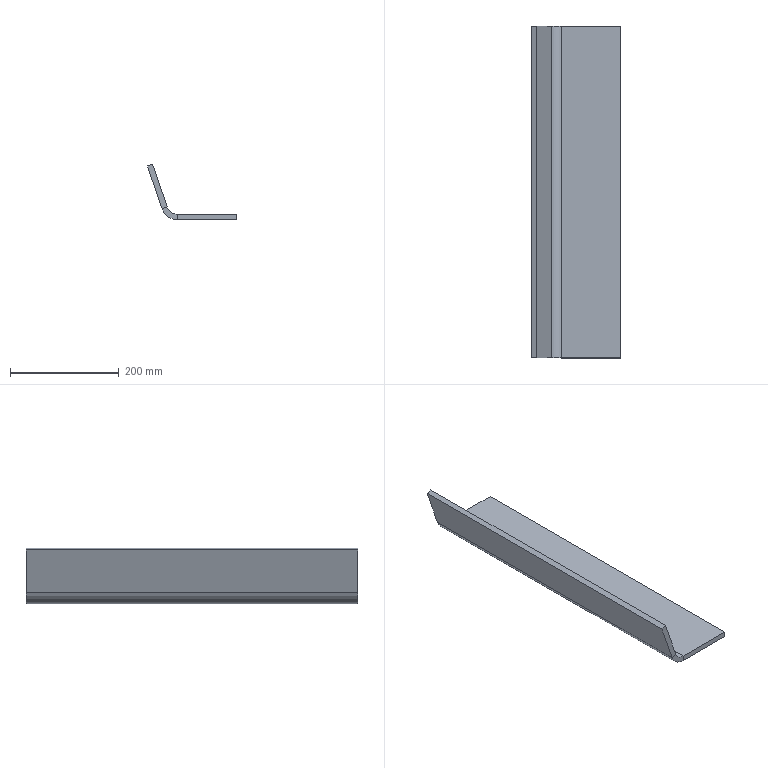Part | SolidWorks | features FlatPattern 1, SM3dBend 1, SMBaseFlange 1, SheetMetal 1 | 1 solid | 14 faces | box 163.637 x 610 x 102.048 mm | volume 1357250 mm3 | plane 12 | cylinder 2 | commonest cylinder face diameters 40 x1 60 x1
STEP:
#1=CARTESIAN_POINT('',(95.05,610.,13.555));
#2=VERTEX_POINT('',#1);
#3=CARTESIAN_POINT('',(68.329,610.,92.048));
#4=VERTEX_POINT('',#3);
#5=CARTESIAN_POINT('',(68.329,610.,92.048));
#6=DIRECTION('',(-0.3223,0.,0.9466));
#7=VECTOR('',#6,1000.);
#8=LINE('',#5,#7);
#9=EDGE_CURVE('',#2,#4,#8,.T.);
#10=ORIENTED_EDGE('',*,*,#9,.F.);
#11=CARTESIAN_POINT('',(85.584,610.,10.332));
#12=VERTEX_POINT('',#11);
#13=CARTESIAN_POINT('',(85.584,610.,10.332));
#14=DIRECTION('',(-0.9466,0.,-0.3223));
#15=VECTOR('',#14,1000.);
#16=LINE('',#13,#15);
#17=EDGE_CURVE('',#2,#12,#16,.T.);
#18=ORIENTED_EDGE('',*,*,#17,.T.);
#19=CARTESIAN_POINT('',(58.863,610.,88.825));
#20=VERTEX_POINT('',#19);
#21=CARTESIAN_POINT('',(58.863,610.,88.825));
#22=DIRECTION('',(-0.3223,0.,0.9466));
#23=VECTOR('',#22,1000.);
#24=LINE('',#21,#23);
#25=EDGE_CURVE('',#12,#20,#24,.T.);
#26=ORIENTED_EDGE('',*,*,#25,.T.);
#27=CARTESIAN_POINT('',(58.863,610.,88.825));
#28=DIRECTION('',(0.9466,0.,0.3223));
#29=VECTOR('',#28,1000.);
#30=LINE('',#27,#29);
#31=EDGE_CURVE('',#20,#4,#30,.T.);
#32=ORIENTED_EDGE('',*,*,#31,.T.);
#33=EDGE_LOOP('',(#10,#18,#26,#32));
#34=FACE_OUTER_BOUND('',#33,.T.);
#35=CARTESIAN_POINT('',(58.863,610.,88.825));
#36=DIRECTION('',(0.,1.,0.));
#37=DIRECTION('',(0.9466,0.,0.3223));
#38=AXIS2_PLACEMENT_3D('',#35,#36,#37);
#39=PLANE('',#38);
#40=ADVANCED_FACE('',(#34),#39,.T.);
#41=CARTESIAN_POINT('',(58.863,0.,88.825));
#42=VERTEX_POINT('',#41);
#43=CARTESIAN_POINT('',(85.584,0.,10.332));
#44=VERTEX_POINT('',#43);
#45=CARTESIAN_POINT('',(58.863,0.,88.825));
#46=DIRECTION('',(0.3223,0.,-0.9466));
#47=VECTOR('',#46,1000.);
#48=LINE('',#45,#47);
#49=EDGE_CURVE('',#42,#44,#48,.T.);
#50=ORIENTED_EDGE('',*,*,#49,.T.);
#51=CARTESIAN_POINT('',(95.05,0.,13.555));
#52=VERTEX_POINT('',#51);
#53=CARTESIAN_POINT('',(85.584,0.,10.332));
#54=DIRECTION('',(0.9466,0.,0.3223));
#55=VECTOR('',#54,1000.);
#56=LINE('',#53,#55);
#57=EDGE_CURVE('',#44,#52,#56,.T.);
#58=ORIENTED_EDGE('',*,*,#57,.T.);
#59=CARTESIAN_POINT('',(68.329,0.,92.048));
#60=VERTEX_POINT('',#59);
#61=CARTESIAN_POINT('',(68.329,0.,92.048));
#62=DIRECTION('',(0.3223,0.,-0.9466));
#63=VECTOR('',#62,1000.);
#64=LINE('',#61,#63);
#65=EDGE_CURVE('',#60,#52,#64,.T.);
#66=ORIENTED_EDGE('',*,*,#65,.F.);
#67=CARTESIAN_POINT('',(58.863,0.,88.825));
#68=DIRECTION('',(0.9466,0.,0.3223));
#69=VECTOR('',#68,1000.);
#70=LINE('',#67,#69);
#71=EDGE_CURVE('',#42,#60,#70,.T.);
#72=ORIENTED_EDGE('',*,*,#71,.F.);
#73=EDGE_LOOP('',(#50,#58,#66,#72));
#74=FACE_OUTER_BOUND('',#73,.T.);
#75=CARTESIAN_POINT('',(58.863,0.,88.825));
#76=DIRECTION('',(0.,-1.,0.));
#77=DIRECTION('',(-0.9466,0.,-0.3223));
#78=AXIS2_PLACEMENT_3D('',#75,#76,#77);
#79=PLANE('',#78);
#80=ADVANCED_FACE('',(#74),#79,.T.);
#81=ORIENTED_EDGE('',*,*,#25,.F.);
#82=CARTESIAN_POINT('',(85.584,610.,10.332));
#83=DIRECTION('',(0.,-1.,0.));
#84=VECTOR('',#83,1000.);
#85=LINE('',#82,#84);
#86=EDGE_CURVE('',#12,#44,#85,.T.);
#87=ORIENTED_EDGE('',*,*,#86,.T.);
#88=ORIENTED_EDGE('',*,*,#49,.F.);
#89=CARTESIAN_POINT('',(58.863,0.,88.825));
#90=DIRECTION('',(0.,-1.,0.));
#91=VECTOR('',#90,1000.);
#92=LINE('',#89,#91);
#93=EDGE_CURVE('',#20,#42,#92,.T.);
#94=ORIENTED_EDGE('',*,*,#93,.F.);
#95=EDGE_LOOP('',(#81,#87,#88,#94));
#96=FACE_OUTER_BOUND('',#95,.T.);
#97=CARTESIAN_POINT('',(58.863,610.,88.825));
#98=DIRECTION('',(-0.9466,0.,-0.3223));
#99=DIRECTION('',(-0.3223,0.,0.9466));
#100=AXIS2_PLACEMENT_3D('',#97,#98,#99);
#101=PLANE('',#100);
#102=ADVANCED_FACE('',(#96),#101,.T.);
#103=CARTESIAN_POINT('',(68.329,0.,92.048));
#104=DIRECTION('',(0.,-1.,0.));
#105=VECTOR('',#104,1000.);
#106=LINE('',#103,#105);
#107=EDGE_CURVE('',#4,#60,#106,.T.);
#108=ORIENTED_EDGE('',*,*,#107,.F.);
#109=ORIENTED_EDGE('',*,*,#31,.F.);
#110=ORIENTED_EDGE('',*,*,#93,.T.);
#111=ORIENTED_EDGE('',*,*,#71,.T.);
#112=EDGE_LOOP('',(#108,#109,#110,#111));
#113=FACE_OUTER_BOUND('',#112,.T.);
#114=CARTESIAN_POINT('',(58.863,0.,88.825));
#115=DIRECTION('',(-0.3223,0.,0.9466));
#116=DIRECTION('',(0.9466,0.,0.3223));
#117=AXIS2_PLACEMENT_3D('',#114,#115,#116);
#118=PLANE('',#117);
#119=ADVANCED_FACE('',(#113),#118,.T.);
#120=CARTESIAN_POINT('',(95.05,610.,13.555));
#121=DIRECTION('',(0.,-1.,0.));
#122=VECTOR('',#121,1000.);
#123=LINE('',#120,#122);
#124=EDGE_CURVE('',#2,#52,#123,.T.);
#125=ORIENTED_EDGE('',*,*,#124,.F.);
#126=ORIENTED_EDGE('',*,*,#9,.T.);
#127=ORIENTED_EDGE('',*,*,#107,.T.);
#128=ORIENTED_EDGE('',*,*,#65,.T.);
#129=EDGE_LOOP('',(#125,#126,#127,#128));
#130=FACE_OUTER_BOUND('',#129,.T.);
#131=CARTESIAN_POINT('',(68.329,610.,92.048));
#132=DIRECTION('',(-0.9466,0.,-0.3223));
#133=DIRECTION('',(-0.3223,0.,0.9466));
#134=AXIS2_PLACEMENT_3D('',#131,#132,#133);
#135=PLANE('',#134);
#136=ADVANCED_FACE('',(#130),#135,.F.);
#137=CARTESIAN_POINT('',(222.5,0.,0.));
#138=VERTEX_POINT('',#137);
#139=CARTESIAN_POINT('',(222.5,610.,0.));
#140=VERTEX_POINT('',#139);
#141=CARTESIAN_POINT('',(222.5,0.,0.));
#142=DIRECTION('',(0.,1.,0.));
#143=VECTOR('',#142,1000.);
#144=LINE('',#141,#143);
#145=EDGE_CURVE('',#138,#140,#144,.T.);
#146=ORIENTED_EDGE('',*,*,#145,.F.);
#147=CARTESIAN_POINT('',(222.5,0.,-10.));
#148=VERTEX_POINT('',#147);
#149=CARTESIAN_POINT('',(222.5,0.,-10.));
#150=DIRECTION('',(0.,0.,1.));
#151=VECTOR('',#150,1000.);
#152=LINE('',#149,#151);
#153=EDGE_CURVE('',#148,#138,#152,.T.);
#154=ORIENTED_EDGE('',*,*,#153,.F.);
#155=CARTESIAN_POINT('',(222.5,610.,-10.));
#156=VERTEX_POINT('',#155);
#157=CARTESIAN_POINT('',(222.5,0.,-10.));
#158=DIRECTION('',(0.,1.,0.));
#159=VECTOR('',#158,1000.);
#160=LINE('',#157,#159);
#161=EDGE_CURVE('',#148,#156,#160,.T.);
#162=ORIENTED_EDGE('',*,*,#161,.T.);
#163=CARTESIAN_POINT('',(222.5,610.,-10.));
#164=DIRECTION('',(0.,0.,1.));
#165=VECTOR('',#164,1000.);
#166=LINE('',#163,#165);
#167=EDGE_CURVE('',#156,#140,#166,.T.);
#168=ORIENTED_EDGE('',*,*,#167,.T.);
#169=EDGE_LOOP('',(#146,#154,#162,#168));
#170=FACE_OUTER_BOUND('',#169,.T.);
#171=CARTESIAN_POINT('',(222.5,0.,-10.));
#172=DIRECTION('',(1.,0.,0.));
#173=DIRECTION('',(0.,0.,-1.));
#174=AXIS2_PLACEMENT_3D('',#171,#172,#173);
#175=PLANE('',#174);
#176=ADVANCED_FACE('',(#170),#175,.T.);
#177=CARTESIAN_POINT('',(113.983,610.,-10.));
#178=VERTEX_POINT('',#177);
#179=CARTESIAN_POINT('',(113.983,0.,-10.));
#180=VERTEX_POINT('',#179);
#181=CARTESIAN_POINT('',(113.983,610.,-10.));
#182=DIRECTION('',(0.,-1.,0.));
#183=VECTOR('',#182,1000.);
#184=LINE('',#181,#183);
#185=EDGE_CURVE('',#178,#180,#184,.T.);
#186=ORIENTED_EDGE('',*,*,#185,.F.);
#187=CARTESIAN_POINT('',(0.,610.,-10.));
#188=DIRECTION('',(-1.,0.,0.));
#189=VECTOR('',#188,1000.);
#190=LINE('',#187,#189);
#191=EDGE_CURVE('',#156,#178,#190,.T.);
#192=ORIENTED_EDGE('',*,*,#191,.F.);
#193=ORIENTED_EDGE('',*,*,#161,.F.);
#194=CARTESIAN_POINT('',(0.,0.,-10.));
#195=DIRECTION('',(1.,0.,0.));
#196=VECTOR('',#195,1000.);
#197=LINE('',#194,#196);
#198=EDGE_CURVE('',#180,#148,#197,.T.);
#199=ORIENTED_EDGE('',*,*,#198,.F.);
#200=EDGE_LOOP('',(#186,#192,#193,#199));
#201=FACE_OUTER_BOUND('',#200,.T.);
#202=CARTESIAN_POINT('',(0.,610.,-10.));
#203=DIRECTION('',(0.,0.,-1.));
#204=DIRECTION('',(-1.,0.,0.));
#205=AXIS2_PLACEMENT_3D('',#202,#203,#204);
#206=PLANE('',#205);
#207=ADVANCED_FACE('',(#201),#206,.T.);
#208=CARTESIAN_POINT('',(113.983,610.,0.));
#209=VERTEX_POINT('',#208);
#210=CARTESIAN_POINT('',(113.983,610.,-10.));
#211=DIRECTION('',(0.,0.,-1.));
#212=VECTOR('',#211,1000.);
#213=LINE('',#210,#212);
#214=EDGE_CURVE('',#209,#178,#213,.T.);
#215=ORIENTED_EDGE('',*,*,#214,.F.);
#216=CARTESIAN_POINT('',(0.,610.,0.));
#217=DIRECTION('',(-1.,0.,0.));
#218=VECTOR('',#217,1000.);
#219=LINE('',#216,#218);
#220=EDGE_CURVE('',#140,#209,#219,.T.);
#221=ORIENTED_EDGE('',*,*,#220,.F.);
#222=ORIENTED_EDGE('',*,*,#167,.F.);
#223=ORIENTED_EDGE('',*,*,#191,.T.);
#224=EDGE_LOOP('',(#215,#221,#222,#223));
#225=FACE_OUTER_BOUND('',#224,.T.);
#226=CARTESIAN_POINT('',(0.,610.,-10.));
#227=DIRECTION('',(0.,1.,0.));
#228=DIRECTION('',(0.,0.,1.));
#229=AXIS2_PLACEMENT_3D('',#226,#227,#228);
#230=PLANE('',#229);
#231=ADVANCED_FACE('',(#225),#230,.T.);
#232=ORIENTED_EDGE('',*,*,#220,.T.);
#233=CARTESIAN_POINT('',(113.983,0.,0.));
#234=VERTEX_POINT('',#233);
#235=CARTESIAN_POINT('',(113.983,610.,0.));
#236=DIRECTION('',(0.,-1.,0.));
#237=VECTOR('',#236,1000.);
#238=LINE('',#235,#237);
#239=EDGE_CURVE('',#209,#234,#238,.T.);
#240=ORIENTED_EDGE('',*,*,#239,.T.);
#241=CARTESIAN_POINT('',(0.,0.,0.));
#242=DIRECTION('',(1.,0.,0.));
#243=VECTOR('',#242,1000.);
#244=LINE('',#241,#243);
#245=EDGE_CURVE('',#234,#138,#244,.T.);
#246=ORIENTED_EDGE('',*,*,#245,.T.);
#247=ORIENTED_EDGE('',*,*,#145,.T.);
#248=EDGE_LOOP('',(#232,#240,#246,#247));
#249=FACE_OUTER_BOUND('',#248,.T.);
#250=CARTESIAN_POINT('',(0.,610.,0.));
#251=DIRECTION('',(0.,0.,-1.));
#252=DIRECTION('',(-1.,0.,0.));
#253=AXIS2_PLACEMENT_3D('',#250,#251,#252);
#254=PLANE('',#253);
#255=ADVANCED_FACE('',(#249),#254,.F.);
#256=CARTESIAN_POINT('',(113.983,0.,-10.));
#257=DIRECTION('',(0.,0.,1.));
#258=VECTOR('',#257,1000.);
#259=LINE('',#256,#258);
#260=EDGE_CURVE('',#180,#234,#259,.T.);
#261=ORIENTED_EDGE('',*,*,#260,.F.);
#262=ORIENTED_EDGE('',*,*,#198,.T.);
#263=ORIENTED_EDGE('',*,*,#153,.T.);
#264=ORIENTED_EDGE('',*,*,#245,.F.);
#265=EDGE_LOOP('',(#261,#262,#263,#264));
#266=FACE_OUTER_BOUND('',#265,.T.);
#267=CARTESIAN_POINT('',(0.,0.,-10.));
#268=DIRECTION('',(0.,-1.,0.));
#269=DIRECTION('',(0.,0.,-1.));
#270=AXIS2_PLACEMENT_3D('',#267,#268,#269);
#271=PLANE('',#270);
#272=ADVANCED_FACE('',(#266),#271,.T.);
#273=ORIENTED_EDGE('',*,*,#17,.F.);
#274=CARTESIAN_POINT('',(113.983,610.,20.));
#275=DIRECTION('',(0.,-1.,0.));
#276=DIRECTION('',(-1.,0.,0.));
#277=AXIS2_PLACEMENT_3D('',#274,#275,#276);
#278=CIRCLE('',#277,20.);
#279=EDGE_CURVE('',#2,#209,#278,.T.);
#280=ORIENTED_EDGE('',*,*,#279,.T.);
#281=ORIENTED_EDGE('',*,*,#214,.T.);
#282=CARTESIAN_POINT('',(113.983,610.,20.));
#283=DIRECTION('',(0.,-1.,0.));
#284=DIRECTION('',(0.,0.,1.));
#285=AXIS2_PLACEMENT_3D('',#282,#283,#284);
#286=CIRCLE('',#285,30.);
#287=EDGE_CURVE('',#12,#178,#286,.T.);
#288=ORIENTED_EDGE('',*,*,#287,.F.);
#289=EDGE_LOOP('',(#273,#280,#281,#288));
#290=FACE_OUTER_BOUND('',#289,.T.);
#291=CARTESIAN_POINT('',(113.983,610.,20.));
#292=DIRECTION('',(0.,1.,0.));
#293=DIRECTION('',(0.,0.,1.));
#294=AXIS2_PLACEMENT_3D('',#291,#292,#293);
#295=PLANE('',#294);
#296=ADVANCED_FACE('',(#290),#295,.T.);
#297=ORIENTED_EDGE('',*,*,#185,.T.);
#298=CARTESIAN_POINT('',(113.983,0.,20.));
#299=DIRECTION('',(0.,1.,0.));
#300=DIRECTION('',(1.,0.,0.));
#301=AXIS2_PLACEMENT_3D('',#298,#299,#300);
#302=CIRCLE('',#301,30.);
#303=EDGE_CURVE('',#180,#44,#302,.T.);
#304=ORIENTED_EDGE('',*,*,#303,.T.);
#305=ORIENTED_EDGE('',*,*,#86,.F.);
#306=ORIENTED_EDGE('',*,*,#287,.T.);
#307=EDGE_LOOP('',(#297,#304,#305,#306));
#308=FACE_OUTER_BOUND('',#307,.T.);
#309=CARTESIAN_POINT('',(113.983,-305.872,20.));
#310=DIRECTION('',(0.,1.,0.));
#311=DIRECTION('',(-1.,0.,0.));
#312=AXIS2_PLACEMENT_3D('',#309,#310,#311);
#313=CYLINDRICAL_SURFACE('',#312,30.);
#314=ADVANCED_FACE('',(#308),#313,.T.);
#315=CARTESIAN_POINT('',(113.983,0.,20.));
#316=DIRECTION('',(0.,1.,0.));
#317=DIRECTION('',(-1.,0.,0.));
#318=AXIS2_PLACEMENT_3D('',#315,#316,#317);
#319=CIRCLE('',#318,20.);
#320=EDGE_CURVE('',#234,#52,#319,.T.);
#321=ORIENTED_EDGE('',*,*,#320,.T.);
#322=ORIENTED_EDGE('',*,*,#57,.F.);
#323=ORIENTED_EDGE('',*,*,#303,.F.);
#324=ORIENTED_EDGE('',*,*,#260,.T.);
#325=EDGE_LOOP('',(#321,#322,#323,#324));
#326=FACE_OUTER_BOUND('',#325,.T.);
#327=CARTESIAN_POINT('',(113.983,0.,20.));
#328=DIRECTION('',(0.,-1.,0.));
#329=DIRECTION('',(1.,0.,0.));
#330=AXIS2_PLACEMENT_3D('',#327,#328,#329);
#331=PLANE('',#330);
#332=ADVANCED_FACE('',(#326),#331,.T.);
#333=ORIENTED_EDGE('',*,*,#239,.F.);
#334=ORIENTED_EDGE('',*,*,#279,.F.);
#335=ORIENTED_EDGE('',*,*,#124,.T.);
#336=ORIENTED_EDGE('',*,*,#320,.F.);
#337=EDGE_LOOP('',(#333,#334,#335,#336));
#338=FACE_OUTER_BOUND('',#337,.T.);
#339=CARTESIAN_POINT('',(113.983,-305.872,20.));
#340=DIRECTION('',(0.,1.,0.));
#341=DIRECTION('',(-1.,0.,0.));
#342=AXIS2_PLACEMENT_3D('',#339,#340,#341);
#343=CYLINDRICAL_SURFACE('',#342,20.);
#344=ADVANCED_FACE('',(#338),#343,.F.);
#345=CLOSED_SHELL('',(#40,#80,#102,#119,#136,#176,#207,#231,#255,#272,#296,#314,#332,#344));
#346=MANIFOLD_SOLID_BREP('',#345);
#347=CARTESIAN_POINT('',(0.,0.,0.));
#348=DIRECTION('',(0.,0.,1.));
#349=DIRECTION('',(1.,0.,0.));
#350=AXIS2_PLACEMENT_3D('',#347,#348,#349);
#351=(LENGTH_UNIT()NAMED_UNIT(*)SI_UNIT(.MILLI.,.METRE.));
#352=UNCERTAINTY_MEASURE_WITH_UNIT(LENGTH_MEASURE(0.00001),#351,'','');
#353=(NAMED_UNIT(*)PLANE_ANGLE_UNIT()SI_UNIT($,.RADIAN.));
#354=(NAMED_UNIT(*)SI_UNIT($,.STERADIAN.)SOLID_ANGLE_UNIT());
#355=(GEOMETRIC_REPRESENTATION_CONTEXT(3)GLOBAL_UNCERTAINTY_ASSIGNED_CONTEXT((#352))GLOBAL_UNIT_ASSIGNED_CONTEXT((#351,#353,#354))REPRESENTATION_CONTEXT('',''));
#356=ADVANCED_BREP_SHAPE_REPRESENTATION('',(#346,#350),#355);